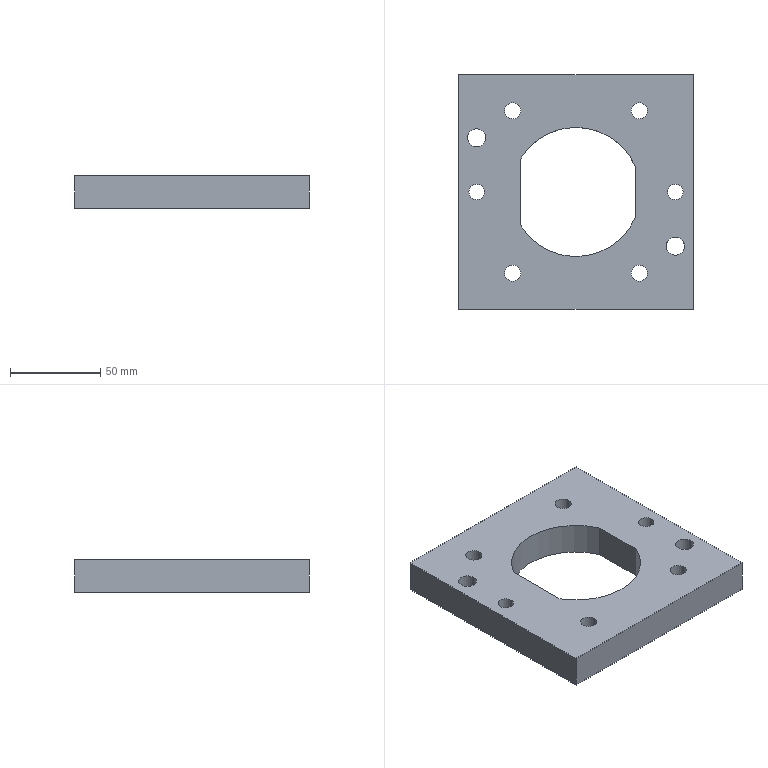Part | SolidWorks | features BaseBody 1 | 1 solid | 30 faces | box 130 x 130 x 18 mm | volume 225680 mm3 | cylinder 18 | plane 8 | cone 4 | commonest cylinder face diameters 9 x8 8.506 x4 10 x4 71.52 x2
STEP:
#1=CARTESIAN_POINT('',(-136.,5.,-28.7));
#2=VERTEX_POINT('',#1);
#3=CARTESIAN_POINT('',(-146.,5.,-28.7));
#4=VERTEX_POINT('',#3);
#5=CARTESIAN_POINT('',(-141.,5.,-28.7));
#6=DIRECTION('',(0.,0.,-1.));
#7=DIRECTION('',(-1.,0.,0.));
#8=AXIS2_PLACEMENT_3D('',#5,#6,#7);
#9=CIRCLE('',#8,5.);
#10=EDGE_CURVE('',#2,#4,#9,.T.);
#11=ORIENTED_EDGE('',*,*,#10,.F.);
#12=CARTESIAN_POINT('',(-136.,5.,-46.7));
#13=VERTEX_POINT('',#12);
#14=CARTESIAN_POINT('',(-136.,5.,-28.7));
#15=DIRECTION('',(0.,0.,-1.));
#16=VECTOR('',#15,1000.);
#17=LINE('',#14,#16);
#18=EDGE_CURVE('',#2,#13,#17,.T.);
#19=ORIENTED_EDGE('',*,*,#18,.T.);
#20=CARTESIAN_POINT('',(-146.,5.,-46.7));
#21=VERTEX_POINT('',#20);
#22=CARTESIAN_POINT('',(-141.,5.,-46.7));
#23=DIRECTION('',(0.,0.,-1.));
#24=DIRECTION('',(-1.,0.,0.));
#25=AXIS2_PLACEMENT_3D('',#22,#23,#24);
#26=CIRCLE('',#25,5.);
#27=EDGE_CURVE('',#13,#21,#26,.T.);
#28=ORIENTED_EDGE('',*,*,#27,.T.);
#29=CARTESIAN_POINT('',(-146.,5.,-28.7));
#30=DIRECTION('',(0.,0.,-1.));
#31=VECTOR('',#30,1000.);
#32=LINE('',#29,#31);
#33=EDGE_CURVE('',#4,#21,#32,.T.);
#34=ORIENTED_EDGE('',*,*,#33,.F.);
#35=EDGE_LOOP('',(#11,#19,#28,#34));
#36=FACE_OUTER_BOUND('',#35,.T.);
#37=CARTESIAN_POINT('',(-141.,5.,-28.7));
#38=DIRECTION('',(0.,0.,-1.));
#39=DIRECTION('',(-1.,0.,0.));
#40=AXIS2_PLACEMENT_3D('',#37,#38,#39);
#41=CYLINDRICAL_SURFACE('',#40,5.);
#42=ADVANCED_FACE('',(#36),#41,.F.);
#43=CARTESIAN_POINT('',(-26.,-55.,-28.7));
#44=VERTEX_POINT('',#43);
#45=CARTESIAN_POINT('',(-36.,-55.,-28.7));
#46=VERTEX_POINT('',#45);
#47=CARTESIAN_POINT('',(-31.,-55.,-28.7));
#48=DIRECTION('',(0.,0.,-1.));
#49=DIRECTION('',(-1.,0.,0.));
#50=AXIS2_PLACEMENT_3D('',#47,#48,#49);
#51=CIRCLE('',#50,5.);
#52=EDGE_CURVE('',#44,#46,#51,.T.);
#53=ORIENTED_EDGE('',*,*,#52,.F.);
#54=CARTESIAN_POINT('',(-26.,-55.,-46.7));
#55=VERTEX_POINT('',#54);
#56=CARTESIAN_POINT('',(-26.,-55.,-28.7));
#57=DIRECTION('',(0.,0.,-1.));
#58=VECTOR('',#57,1000.);
#59=LINE('',#56,#58);
#60=EDGE_CURVE('',#44,#55,#59,.T.);
#61=ORIENTED_EDGE('',*,*,#60,.T.);
#62=CARTESIAN_POINT('',(-36.,-55.,-46.7));
#63=VERTEX_POINT('',#62);
#64=CARTESIAN_POINT('',(-31.,-55.,-46.7));
#65=DIRECTION('',(0.,0.,-1.));
#66=DIRECTION('',(-1.,0.,0.));
#67=AXIS2_PLACEMENT_3D('',#64,#65,#66);
#68=CIRCLE('',#67,5.);
#69=EDGE_CURVE('',#55,#63,#68,.T.);
#70=ORIENTED_EDGE('',*,*,#69,.T.);
#71=CARTESIAN_POINT('',(-36.,-55.,-28.7));
#72=DIRECTION('',(0.,0.,-1.));
#73=VECTOR('',#72,1000.);
#74=LINE('',#71,#73);
#75=EDGE_CURVE('',#46,#63,#74,.T.);
#76=ORIENTED_EDGE('',*,*,#75,.F.);
#77=EDGE_LOOP('',(#53,#61,#70,#76));
#78=FACE_OUTER_BOUND('',#77,.T.);
#79=CARTESIAN_POINT('',(-31.,-55.,-28.7));
#80=DIRECTION('',(0.,0.,-1.));
#81=DIRECTION('',(-1.,0.,0.));
#82=AXIS2_PLACEMENT_3D('',#79,#80,#81);
#83=CYLINDRICAL_SURFACE('',#82,5.);
#84=ADVANCED_FACE('',(#78),#83,.F.);
#85=CARTESIAN_POINT('',(-145.253,-25.,-45.953));
#86=VERTEX_POINT('',#85);
#87=CARTESIAN_POINT('',(-136.747,-25.,-45.953));
#88=VERTEX_POINT('',#87);
#89=CARTESIAN_POINT('',(-141.,-25.,-45.953));
#90=DIRECTION('',(0.,0.,1.));
#91=DIRECTION('',(-1.,0.,0.));
#92=AXIS2_PLACEMENT_3D('',#89,#90,#91);
#93=CIRCLE('',#92,4.253);
#94=EDGE_CURVE('',#86,#88,#93,.T.);
#95=ORIENTED_EDGE('',*,*,#94,.T.);
#96=CARTESIAN_POINT('',(-136.,-25.,-46.7));
#97=VERTEX_POINT('',#96);
#98=CARTESIAN_POINT('',(-136.,-25.,-46.7));
#99=DIRECTION('',(0.7071,0.,-0.7071));
#100=VECTOR('',#99,1000.);
#101=LINE('',#98,#100);
#102=EDGE_CURVE('',#88,#97,#101,.T.);
#103=ORIENTED_EDGE('',*,*,#102,.T.);
#104=CARTESIAN_POINT('',(-146.,-25.,-46.7));
#105=VERTEX_POINT('',#104);
#106=CARTESIAN_POINT('',(-141.,-25.,-46.7));
#107=DIRECTION('',(0.,0.,-1.));
#108=DIRECTION('',(-1.,0.,0.));
#109=AXIS2_PLACEMENT_3D('',#106,#107,#108);
#110=CIRCLE('',#109,5.);
#111=EDGE_CURVE('',#97,#105,#110,.T.);
#112=ORIENTED_EDGE('',*,*,#111,.T.);
#113=CARTESIAN_POINT('',(-146.,-25.,-46.7));
#114=DIRECTION('',(-0.7071,0.,-0.7071));
#115=VECTOR('',#114,1000.);
#116=LINE('',#113,#115);
#117=EDGE_CURVE('',#86,#105,#116,.T.);
#118=ORIENTED_EDGE('',*,*,#117,.F.);
#119=EDGE_LOOP('',(#95,#103,#112,#118));
#120=FACE_OUTER_BOUND('',#119,.T.);
#121=CARTESIAN_POINT('',(-141.,-25.,-46.7));
#122=DIRECTION('',(0.,0.,-1.));
#123=DIRECTION('',(-1.,0.,0.));
#124=AXIS2_PLACEMENT_3D('',#121,#122,#123);
#125=CONICAL_SURFACE('',#124,5.,0.7854);
#126=ADVANCED_FACE('',(#120),#125,.F.);
#127=CARTESIAN_POINT('',(-136.747,-25.,-28.7));
#128=VERTEX_POINT('',#127);
#129=CARTESIAN_POINT('',(-145.253,-25.,-28.7));
#130=VERTEX_POINT('',#129);
#131=CARTESIAN_POINT('',(-141.,-25.,-28.7));
#132=DIRECTION('',(0.,0.,-1.));
#133=DIRECTION('',(-1.,0.,0.));
#134=AXIS2_PLACEMENT_3D('',#131,#132,#133);
#135=CIRCLE('',#134,4.253);
#136=EDGE_CURVE('',#128,#130,#135,.T.);
#137=ORIENTED_EDGE('',*,*,#136,.F.);
#138=CARTESIAN_POINT('',(-136.747,-25.,-11.867));
#139=DIRECTION('',(0.,0.,-1.));
#140=VECTOR('',#139,1000.);
#141=LINE('',#138,#140);
#142=EDGE_CURVE('',#128,#88,#141,.T.);
#143=ORIENTED_EDGE('',*,*,#142,.T.);
#144=ORIENTED_EDGE('',*,*,#94,.F.);
#145=CARTESIAN_POINT('',(-145.253,-25.,-11.867));
#146=DIRECTION('',(0.,0.,-1.));
#147=VECTOR('',#146,1000.);
#148=LINE('',#145,#147);
#149=EDGE_CURVE('',#130,#86,#148,.T.);
#150=ORIENTED_EDGE('',*,*,#149,.F.);
#151=EDGE_LOOP('',(#137,#143,#144,#150));
#152=FACE_OUTER_BOUND('',#151,.T.);
#153=CARTESIAN_POINT('',(-141.,-25.,-11.867));
#154=DIRECTION('',(0.,0.,-1.));
#155=DIRECTION('',(-1.,0.,0.));
#156=AXIS2_PLACEMENT_3D('',#153,#154,#155);
#157=CYLINDRICAL_SURFACE('',#156,4.253);
#158=ADVANCED_FACE('',(#152),#157,.F.);
#159=CARTESIAN_POINT('',(-35.253,-25.,-45.953));
#160=VERTEX_POINT('',#159);
#161=CARTESIAN_POINT('',(-26.747,-25.,-45.953));
#162=VERTEX_POINT('',#161);
#163=CARTESIAN_POINT('',(-31.,-25.,-45.953));
#164=DIRECTION('',(0.,0.,1.));
#165=DIRECTION('',(-1.,0.,0.));
#166=AXIS2_PLACEMENT_3D('',#163,#164,#165);
#167=CIRCLE('',#166,4.253);
#168=EDGE_CURVE('',#160,#162,#167,.T.);
#169=ORIENTED_EDGE('',*,*,#168,.T.);
#170=CARTESIAN_POINT('',(-26.,-25.,-46.7));
#171=VERTEX_POINT('',#170);
#172=CARTESIAN_POINT('',(-26.,-25.,-46.7));
#173=DIRECTION('',(0.7071,0.,-0.7071));
#174=VECTOR('',#173,1000.);
#175=LINE('',#172,#174);
#176=EDGE_CURVE('',#162,#171,#175,.T.);
#177=ORIENTED_EDGE('',*,*,#176,.T.);
#178=CARTESIAN_POINT('',(-36.,-25.,-46.7));
#179=VERTEX_POINT('',#178);
#180=CARTESIAN_POINT('',(-31.,-25.,-46.7));
#181=DIRECTION('',(0.,0.,-1.));
#182=DIRECTION('',(-1.,0.,0.));
#183=AXIS2_PLACEMENT_3D('',#180,#181,#182);
#184=CIRCLE('',#183,5.);
#185=EDGE_CURVE('',#171,#179,#184,.T.);
#186=ORIENTED_EDGE('',*,*,#185,.T.);
#187=CARTESIAN_POINT('',(-36.,-25.,-46.7));
#188=DIRECTION('',(-0.7071,0.,-0.7071));
#189=VECTOR('',#188,1000.);
#190=LINE('',#187,#189);
#191=EDGE_CURVE('',#160,#179,#190,.T.);
#192=ORIENTED_EDGE('',*,*,#191,.F.);
#193=EDGE_LOOP('',(#169,#177,#186,#192));
#194=FACE_OUTER_BOUND('',#193,.T.);
#195=CARTESIAN_POINT('',(-31.,-25.,-46.7));
#196=DIRECTION('',(0.,0.,-1.));
#197=DIRECTION('',(-1.,0.,0.));
#198=AXIS2_PLACEMENT_3D('',#195,#196,#197);
#199=CONICAL_SURFACE('',#198,5.,0.7854);
#200=ADVANCED_FACE('',(#194),#199,.F.);
#201=CARTESIAN_POINT('',(-26.747,-25.,-28.7));
#202=VERTEX_POINT('',#201);
#203=CARTESIAN_POINT('',(-35.253,-25.,-28.7));
#204=VERTEX_POINT('',#203);
#205=CARTESIAN_POINT('',(-31.,-25.,-28.7));
#206=DIRECTION('',(0.,0.,-1.));
#207=DIRECTION('',(-1.,0.,0.));
#208=AXIS2_PLACEMENT_3D('',#205,#206,#207);
#209=CIRCLE('',#208,4.253);
#210=EDGE_CURVE('',#202,#204,#209,.T.);
#211=ORIENTED_EDGE('',*,*,#210,.F.);
#212=CARTESIAN_POINT('',(-26.747,-25.,-11.867));
#213=DIRECTION('',(0.,0.,-1.));
#214=VECTOR('',#213,1000.);
#215=LINE('',#212,#214);
#216=EDGE_CURVE('',#202,#162,#215,.T.);
#217=ORIENTED_EDGE('',*,*,#216,.T.);
#218=ORIENTED_EDGE('',*,*,#168,.F.);
#219=CARTESIAN_POINT('',(-35.253,-25.,-11.867));
#220=DIRECTION('',(0.,0.,-1.));
#221=VECTOR('',#220,1000.);
#222=LINE('',#219,#221);
#223=EDGE_CURVE('',#204,#160,#222,.T.);
#224=ORIENTED_EDGE('',*,*,#223,.F.);
#225=EDGE_LOOP('',(#211,#217,#218,#224));
#226=FACE_OUTER_BOUND('',#225,.T.);
#227=CARTESIAN_POINT('',(-31.,-25.,-11.867));
#228=DIRECTION('',(0.,0.,-1.));
#229=DIRECTION('',(-1.,0.,0.));
#230=AXIS2_PLACEMENT_3D('',#227,#228,#229);
#231=CYLINDRICAL_SURFACE('',#230,4.253);
#232=ADVANCED_FACE('',(#226),#231,.F.);
#233=CARTESIAN_POINT('',(-125.5,-70.,-46.7));
#234=VERTEX_POINT('',#233);
#235=CARTESIAN_POINT('',(-116.5,-70.,-46.7));
#236=VERTEX_POINT('',#235);
#237=CARTESIAN_POINT('',(-121.,-70.,-46.7));
#238=DIRECTION('',(0.,0.,-1.));
#239=DIRECTION('',(-1.,0.,0.));
#240=AXIS2_PLACEMENT_3D('',#237,#238,#239);
#241=CIRCLE('',#240,4.5);
#242=EDGE_CURVE('',#234,#236,#241,.T.);
#243=ORIENTED_EDGE('',*,*,#242,.T.);
#244=CARTESIAN_POINT('',(-116.5,-70.,-28.7));
#245=VERTEX_POINT('',#244);
#246=CARTESIAN_POINT('',(-116.5,-70.,-51.7));
#247=DIRECTION('',(0.,0.,1.));
#248=VECTOR('',#247,1000.);
#249=LINE('',#246,#248);
#250=EDGE_CURVE('',#236,#245,#249,.T.);
#251=ORIENTED_EDGE('',*,*,#250,.T.);
#252=CARTESIAN_POINT('',(-125.5,-70.,-28.7));
#253=VERTEX_POINT('',#252);
#254=CARTESIAN_POINT('',(-121.,-70.,-28.7));
#255=DIRECTION('',(0.,0.,-1.));
#256=DIRECTION('',(-1.,0.,0.));
#257=AXIS2_PLACEMENT_3D('',#254,#255,#256);
#258=CIRCLE('',#257,4.5);
#259=EDGE_CURVE('',#253,#245,#258,.T.);
#260=ORIENTED_EDGE('',*,*,#259,.F.);
#261=CARTESIAN_POINT('',(-125.5,-70.,-51.7));
#262=DIRECTION('',(0.,0.,1.));
#263=VECTOR('',#262,1000.);
#264=LINE('',#261,#263);
#265=EDGE_CURVE('',#234,#253,#264,.T.);
#266=ORIENTED_EDGE('',*,*,#265,.F.);
#267=EDGE_LOOP('',(#243,#251,#260,#266));
#268=FACE_OUTER_BOUND('',#267,.T.);
#269=CARTESIAN_POINT('',(-121.,-70.,-51.7));
#270=DIRECTION('',(0.,0.,1.));
#271=DIRECTION('',(-1.,0.,0.));
#272=AXIS2_PLACEMENT_3D('',#269,#270,#271);
#273=CYLINDRICAL_SURFACE('',#272,4.5);
#274=ADVANCED_FACE('',(#268),#273,.F.);
#275=CARTESIAN_POINT('',(-46.5,20.,-46.7));
#276=VERTEX_POINT('',#275);
#277=CARTESIAN_POINT('',(-55.5,20.,-46.7));
#278=VERTEX_POINT('',#277);
#279=CARTESIAN_POINT('',(-51.,20.,-46.7));
#280=DIRECTION('',(0.,0.,-1.));
#281=DIRECTION('',(-1.,0.,0.));
#282=AXIS2_PLACEMENT_3D('',#279,#280,#281);
#283=CIRCLE('',#282,4.5);
#284=EDGE_CURVE('',#276,#278,#283,.T.);
#285=ORIENTED_EDGE('',*,*,#284,.T.);
#286=CARTESIAN_POINT('',(-55.5,20.,-28.7));
#287=VERTEX_POINT('',#286);
#288=CARTESIAN_POINT('',(-55.5,20.,-51.7));
#289=DIRECTION('',(0.,0.,1.));
#290=VECTOR('',#289,1000.);
#291=LINE('',#288,#290);
#292=EDGE_CURVE('',#278,#287,#291,.T.);
#293=ORIENTED_EDGE('',*,*,#292,.T.);
#294=CARTESIAN_POINT('',(-46.5,20.,-28.7));
#295=VERTEX_POINT('',#294);
#296=CARTESIAN_POINT('',(-51.,20.,-28.7));
#297=DIRECTION('',(0.,0.,-1.));
#298=DIRECTION('',(-1.,0.,0.));
#299=AXIS2_PLACEMENT_3D('',#296,#297,#298);
#300=CIRCLE('',#299,4.5);
#301=EDGE_CURVE('',#295,#287,#300,.T.);
#302=ORIENTED_EDGE('',*,*,#301,.F.);
#303=CARTESIAN_POINT('',(-46.5,20.,-51.7));
#304=DIRECTION('',(0.,0.,1.));
#305=VECTOR('',#304,1000.);
#306=LINE('',#303,#305);
#307=EDGE_CURVE('',#276,#295,#306,.T.);
#308=ORIENTED_EDGE('',*,*,#307,.F.);
#309=EDGE_LOOP('',(#285,#293,#302,#308));
#310=FACE_OUTER_BOUND('',#309,.T.);
#311=CARTESIAN_POINT('',(-51.,20.,-51.7));
#312=DIRECTION('',(0.,0.,1.));
#313=DIRECTION('',(1.,0.,0.));
#314=AXIS2_PLACEMENT_3D('',#311,#312,#313);
#315=CYLINDRICAL_SURFACE('',#314,4.5);
#316=ADVANCED_FACE('',(#310),#315,.F.);
#317=CARTESIAN_POINT('',(-116.5,20.,-46.7));
#318=VERTEX_POINT('',#317);
#319=CARTESIAN_POINT('',(-125.5,20.,-46.7));
#320=VERTEX_POINT('',#319);
#321=CARTESIAN_POINT('',(-121.,20.,-46.7));
#322=DIRECTION('',(0.,0.,1.));
#323=DIRECTION('',(-1.,0.,0.));
#324=AXIS2_PLACEMENT_3D('',#321,#322,#323);
#325=CIRCLE('',#324,4.5);
#326=EDGE_CURVE('',#318,#320,#325,.T.);
#327=ORIENTED_EDGE('',*,*,#326,.F.);
#328=CARTESIAN_POINT('',(-116.5,20.,-28.7));
#329=VERTEX_POINT('',#328);
#330=CARTESIAN_POINT('',(-116.5,20.,-51.7));
#331=DIRECTION('',(0.,0.,1.));
#332=VECTOR('',#331,1000.);
#333=LINE('',#330,#332);
#334=EDGE_CURVE('',#318,#329,#333,.T.);
#335=ORIENTED_EDGE('',*,*,#334,.T.);
#336=CARTESIAN_POINT('',(-125.5,20.,-28.7));
#337=VERTEX_POINT('',#336);
#338=CARTESIAN_POINT('',(-121.,20.,-28.7));
#339=DIRECTION('',(0.,0.,-1.));
#340=DIRECTION('',(-1.,0.,0.));
#341=AXIS2_PLACEMENT_3D('',#338,#339,#340);
#342=CIRCLE('',#341,4.5);
#343=EDGE_CURVE('',#337,#329,#342,.T.);
#344=ORIENTED_EDGE('',*,*,#343,.F.);
#345=CARTESIAN_POINT('',(-125.5,20.,-51.7));
#346=DIRECTION('',(0.,0.,1.));
#347=VECTOR('',#346,1000.);
#348=LINE('',#345,#347);
#349=EDGE_CURVE('',#320,#337,#348,.T.);
#350=ORIENTED_EDGE('',*,*,#349,.F.);
#351=EDGE_LOOP('',(#327,#335,#344,#350));
#352=FACE_OUTER_BOUND('',#351,.T.);
#353=CARTESIAN_POINT('',(-121.,20.,-51.7));
#354=DIRECTION('',(0.,0.,1.));
#355=DIRECTION('',(-1.,0.,0.));
#356=AXIS2_PLACEMENT_3D('',#353,#354,#355);
#357=CYLINDRICAL_SURFACE('',#356,4.5);
#358=ADVANCED_FACE('',(#352),#357,.F.);
#359=CARTESIAN_POINT('',(-55.5,-70.,-46.7));
#360=VERTEX_POINT('',#359);
#361=CARTESIAN_POINT('',(-46.5,-70.,-46.7));
#362=VERTEX_POINT('',#361);
#363=CARTESIAN_POINT('',(-51.,-70.,-46.7));
#364=DIRECTION('',(0.,0.,1.));
#365=DIRECTION('',(-1.,0.,0.));
#366=AXIS2_PLACEMENT_3D('',#363,#364,#365);
#367=CIRCLE('',#366,4.5);
#368=EDGE_CURVE('',#360,#362,#367,.T.);
#369=ORIENTED_EDGE('',*,*,#368,.F.);
#370=CARTESIAN_POINT('',(-55.5,-70.,-28.7));
#371=VERTEX_POINT('',#370);
#372=CARTESIAN_POINT('',(-55.5,-70.,-51.7));
#373=DIRECTION('',(0.,0.,1.));
#374=VECTOR('',#373,1000.);
#375=LINE('',#372,#374);
#376=EDGE_CURVE('',#360,#371,#375,.T.);
#377=ORIENTED_EDGE('',*,*,#376,.T.);
#378=CARTESIAN_POINT('',(-46.5,-70.,-28.7));
#379=VERTEX_POINT('',#378);
#380=CARTESIAN_POINT('',(-51.,-70.,-28.7));
#381=DIRECTION('',(0.,0.,-1.));
#382=DIRECTION('',(-1.,0.,0.));
#383=AXIS2_PLACEMENT_3D('',#380,#381,#382);
#384=CIRCLE('',#383,4.5);
#385=EDGE_CURVE('',#379,#371,#384,.T.);
#386=ORIENTED_EDGE('',*,*,#385,.F.);
#387=CARTESIAN_POINT('',(-46.5,-70.,-51.7));
#388=DIRECTION('',(0.,0.,1.));
#389=VECTOR('',#388,1000.);
#390=LINE('',#387,#389);
#391=EDGE_CURVE('',#362,#379,#390,.T.);
#392=ORIENTED_EDGE('',*,*,#391,.F.);
#393=EDGE_LOOP('',(#369,#377,#386,#392));
#394=FACE_OUTER_BOUND('',#393,.T.);
#395=CARTESIAN_POINT('',(-51.,-70.,-51.7));
#396=DIRECTION('',(0.,0.,1.));
#397=DIRECTION('',(1.,0.,0.));
#398=AXIS2_PLACEMENT_3D('',#395,#396,#397);
#399=CYLINDRICAL_SURFACE('',#398,4.5);
#400=ADVANCED_FACE('',(#394),#399,.F.);
#401=CARTESIAN_POINT('',(-141.,5.,-46.7));
#402=DIRECTION('',(0.,0.,-1.));
#403=DIRECTION('',(-1.,0.,0.));
#404=AXIS2_PLACEMENT_3D('',#401,#402,#403);
#405=CIRCLE('',#404,5.);
#406=EDGE_CURVE('',#21,#13,#405,.T.);
#407=ORIENTED_EDGE('',*,*,#406,.F.);
#408=ORIENTED_EDGE('',*,*,#27,.F.);
#409=EDGE_LOOP('',(#407,#408));
#410=FACE_BOUND('',#409,.T.);
#411=CARTESIAN_POINT('',(-151.,-90.,-46.7));
#412=VERTEX_POINT('',#411);
#413=CARTESIAN_POINT('',(-21.,-90.,-46.7));
#414=VERTEX_POINT('',#413);
#415=CARTESIAN_POINT('',(-86.,-90.,-46.7));
#416=DIRECTION('',(1.,0.,0.));
#417=VECTOR('',#416,1000.);
#418=LINE('',#415,#417);
#419=EDGE_CURVE('',#412,#414,#418,.T.);
#420=ORIENTED_EDGE('',*,*,#419,.F.);
#421=CARTESIAN_POINT('',(-151.,40.,-46.7));
#422=VERTEX_POINT('',#421);
#423=CARTESIAN_POINT('',(-151.,-25.,-46.7));
#424=DIRECTION('',(0.,-1.,0.));
#425=VECTOR('',#424,1000.);
#426=LINE('',#423,#425);
#427=EDGE_CURVE('',#422,#412,#426,.T.);
#428=ORIENTED_EDGE('',*,*,#427,.F.);
#429=CARTESIAN_POINT('',(-21.,40.,-46.7));
#430=VERTEX_POINT('',#429);
#431=CARTESIAN_POINT('',(-86.,40.,-46.7));
#432=DIRECTION('',(-1.,0.,0.));
#433=VECTOR('',#432,1000.);
#434=LINE('',#431,#433);
#435=EDGE_CURVE('',#430,#422,#434,.T.);
#436=ORIENTED_EDGE('',*,*,#435,.F.);
#437=CARTESIAN_POINT('',(-21.,-25.,-46.7));
#438=DIRECTION('',(0.,1.,0.));
#439=VECTOR('',#438,1000.);
#440=LINE('',#437,#439);
#441=EDGE_CURVE('',#414,#430,#440,.T.);
#442=ORIENTED_EDGE('',*,*,#441,.F.);
#443=EDGE_LOOP('',(#420,#428,#436,#442));
#444=FACE_OUTER_BOUND('',#443,.T.);
#445=CARTESIAN_POINT('',(-31.,-55.,-46.7));
#446=DIRECTION('',(0.,0.,-1.));
#447=DIRECTION('',(-1.,0.,0.));
#448=AXIS2_PLACEMENT_3D('',#445,#446,#447);
#449=CIRCLE('',#448,5.);
#450=EDGE_CURVE('',#63,#55,#449,.T.);
#451=ORIENTED_EDGE('',*,*,#450,.F.);
#452=ORIENTED_EDGE('',*,*,#69,.F.);
#453=EDGE_LOOP('',(#451,#452));
#454=FACE_BOUND('',#453,.T.);
#455=CARTESIAN_POINT('',(-141.,-25.,-46.7));
#456=DIRECTION('',(0.,0.,-1.));
#457=DIRECTION('',(-1.,0.,0.));
#458=AXIS2_PLACEMENT_3D('',#455,#456,#457);
#459=CIRCLE('',#458,5.);
#460=EDGE_CURVE('',#105,#97,#459,.T.);
#461=ORIENTED_EDGE('',*,*,#460,.F.);
#462=ORIENTED_EDGE('',*,*,#111,.F.);
#463=EDGE_LOOP('',(#461,#462));
#464=FACE_BOUND('',#463,.T.);
#465=CARTESIAN_POINT('',(-31.,-25.,-46.7));
#466=DIRECTION('',(0.,0.,-1.));
#467=DIRECTION('',(-1.,0.,0.));
#468=AXIS2_PLACEMENT_3D('',#465,#466,#467);
#469=CIRCLE('',#468,5.);
#470=EDGE_CURVE('',#179,#171,#469,.T.);
#471=ORIENTED_EDGE('',*,*,#470,.F.);
#472=ORIENTED_EDGE('',*,*,#185,.F.);
#473=EDGE_LOOP('',(#471,#472));
#474=FACE_BOUND('',#473,.T.);
#475=CARTESIAN_POINT('',(-53.24,-10.663,-46.7));
#476=VERTEX_POINT('',#475);
#477=CARTESIAN_POINT('',(-116.76,-6.763,-46.7));
#478=VERTEX_POINT('',#477);
#479=CARTESIAN_POINT('',(-86.,-25.,-46.7));
#480=DIRECTION('',(0.,0.,1.));
#481=DIRECTION('',(-1.,0.,0.));
#482=AXIS2_PLACEMENT_3D('',#479,#480,#481);
#483=CIRCLE('',#482,35.76);
#484=EDGE_CURVE('',#476,#478,#483,.T.);
#485=ORIENTED_EDGE('',*,*,#484,.T.);
#486=CARTESIAN_POINT('',(-116.76,-43.237,-46.7));
#487=VERTEX_POINT('',#486);
#488=CARTESIAN_POINT('',(-116.76,-25.,-46.7));
#489=DIRECTION('',(0.,-1.,0.));
#490=VECTOR('',#489,1000.);
#491=LINE('',#488,#490);
#492=EDGE_CURVE('',#478,#487,#491,.T.);
#493=ORIENTED_EDGE('',*,*,#492,.T.);
#494=CARTESIAN_POINT('',(-53.24,-39.337,-46.7));
#495=VERTEX_POINT('',#494);
#496=CARTESIAN_POINT('',(-86.,-25.,-46.7));
#497=DIRECTION('',(0.,0.,1.));
#498=DIRECTION('',(-1.,0.,0.));
#499=AXIS2_PLACEMENT_3D('',#496,#497,#498);
#500=CIRCLE('',#499,35.76);
#501=EDGE_CURVE('',#487,#495,#500,.T.);
#502=ORIENTED_EDGE('',*,*,#501,.T.);
#503=CARTESIAN_POINT('',(-53.24,-25.,-46.7));
#504=DIRECTION('',(0.,1.,0.));
#505=VECTOR('',#504,1000.);
#506=LINE('',#503,#505);
#507=EDGE_CURVE('',#495,#476,#506,.T.);
#508=ORIENTED_EDGE('',*,*,#507,.T.);
#509=EDGE_LOOP('',(#485,#493,#502,#508));
#510=FACE_BOUND('',#509,.T.);
#511=CARTESIAN_POINT('',(-51.,-70.,-46.7));
#512=DIRECTION('',(0.,0.,1.));
#513=DIRECTION('',(-1.,0.,0.));
#514=AXIS2_PLACEMENT_3D('',#511,#512,#513);
#515=CIRCLE('',#514,4.5);
#516=EDGE_CURVE('',#362,#360,#515,.T.);
#517=ORIENTED_EDGE('',*,*,#516,.T.);
#518=ORIENTED_EDGE('',*,*,#368,.T.);
#519=EDGE_LOOP('',(#517,#518));
#520=FACE_BOUND('',#519,.T.);
#521=ORIENTED_EDGE('',*,*,#284,.F.);
#522=CARTESIAN_POINT('',(-51.,20.,-46.7));
#523=DIRECTION('',(0.,0.,-1.));
#524=DIRECTION('',(-1.,0.,0.));
#525=AXIS2_PLACEMENT_3D('',#522,#523,#524);
#526=CIRCLE('',#525,4.5);
#527=EDGE_CURVE('',#278,#276,#526,.T.);
#528=ORIENTED_EDGE('',*,*,#527,.F.);
#529=EDGE_LOOP('',(#521,#528));
#530=FACE_BOUND('',#529,.T.);
#531=CARTESIAN_POINT('',(-121.,20.,-46.7));
#532=DIRECTION('',(0.,0.,1.));
#533=DIRECTION('',(-1.,0.,0.));
#534=AXIS2_PLACEMENT_3D('',#531,#532,#533);
#535=CIRCLE('',#534,4.5);
#536=EDGE_CURVE('',#320,#318,#535,.T.);
#537=ORIENTED_EDGE('',*,*,#536,.T.);
#538=ORIENTED_EDGE('',*,*,#326,.T.);
#539=EDGE_LOOP('',(#537,#538));
#540=FACE_BOUND('',#539,.T.);
#541=ORIENTED_EDGE('',*,*,#242,.F.);
#542=CARTESIAN_POINT('',(-121.,-70.,-46.7));
#543=DIRECTION('',(0.,0.,-1.));
#544=DIRECTION('',(-1.,0.,0.));
#545=AXIS2_PLACEMENT_3D('',#542,#543,#544);
#546=CIRCLE('',#545,4.5);
#547=EDGE_CURVE('',#236,#234,#546,.T.);
#548=ORIENTED_EDGE('',*,*,#547,.F.);
#549=EDGE_LOOP('',(#541,#548));
#550=FACE_BOUND('',#549,.T.);
#551=CARTESIAN_POINT('',(-86.,-25.,-46.7));
#552=DIRECTION('',(0.,0.,-1.));
#553=DIRECTION('',(-1.,0.,0.));
#554=AXIS2_PLACEMENT_3D('',#551,#552,#553);
#555=PLANE('',#554);
#556=ADVANCED_FACE('',(#410,#444,#454,#464,#474,#510,#520,#530,#540,#550),#555,.T.);
#557=CARTESIAN_POINT('',(-151.,-90.,-28.7));
#558=VERTEX_POINT('',#557);
#559=CARTESIAN_POINT('',(-21.,-90.,-28.7));
#560=VERTEX_POINT('',#559);
#561=CARTESIAN_POINT('',(-86.,-90.,-28.7));
#562=DIRECTION('',(1.,0.,0.));
#563=VECTOR('',#562,1000.);
#564=LINE('',#561,#563);
#565=EDGE_CURVE('',#558,#560,#564,.T.);
#566=ORIENTED_EDGE('',*,*,#565,.F.);
#567=CARTESIAN_POINT('',(-151.,-90.,-8.7));
#568=DIRECTION('',(0.,0.,-1.));
#569=VECTOR('',#568,1000.);
#570=LINE('',#567,#569);
#571=EDGE_CURVE('',#558,#412,#570,.T.);
#572=ORIENTED_EDGE('',*,*,#571,.T.);
#573=ORIENTED_EDGE('',*,*,#419,.T.);
#574=CARTESIAN_POINT('',(-21.,-90.,-8.7));
#575=DIRECTION('',(0.,0.,-1.));
#576=VECTOR('',#575,1000.);
#577=LINE('',#574,#576);
#578=EDGE_CURVE('',#560,#414,#577,.T.);
#579=ORIENTED_EDGE('',*,*,#578,.F.);
#580=EDGE_LOOP('',(#566,#572,#573,#579));
#581=FACE_OUTER_BOUND('',#580,.T.);
#582=CARTESIAN_POINT('',(-86.,-90.,-8.7));
#583=DIRECTION('',(0.,-1.,0.));
#584=DIRECTION('',(0.,0.,1.));
#585=AXIS2_PLACEMENT_3D('',#582,#583,#584);
#586=PLANE('',#585);
#587=ADVANCED_FACE('',(#581),#586,.T.);
#588=CARTESIAN_POINT('',(-21.,40.,-28.7));
#589=VERTEX_POINT('',#588);
#590=CARTESIAN_POINT('',(-21.,-25.,-28.7));
#591=DIRECTION('',(0.,1.,0.));
#592=VECTOR('',#591,1000.);
#593=LINE('',#590,#592);
#594=EDGE_CURVE('',#560,#589,#593,.T.);
#595=ORIENTED_EDGE('',*,*,#594,.F.);
#596=ORIENTED_EDGE('',*,*,#578,.T.);
#597=ORIENTED_EDGE('',*,*,#441,.T.);
#598=CARTESIAN_POINT('',(-21.,40.,-8.7));
#599=DIRECTION('',(0.,0.,-1.));
#600=VECTOR('',#599,1000.);
#601=LINE('',#598,#600);
#602=EDGE_CURVE('',#589,#430,#601,.T.);
#603=ORIENTED_EDGE('',*,*,#602,.F.);
#604=EDGE_LOOP('',(#595,#596,#597,#603));
#605=FACE_OUTER_BOUND('',#604,.T.);
#606=CARTESIAN_POINT('',(-21.,-25.,-8.7));
#607=DIRECTION('',(1.,0.,0.));
#608=DIRECTION('',(0.,0.,-1.));
#609=AXIS2_PLACEMENT_3D('',#606,#607,#608);
#610=PLANE('',#609);
#611=ADVANCED_FACE('',(#605),#610,.T.);
#612=CARTESIAN_POINT('',(-151.,40.,-28.7));
#613=VERTEX_POINT('',#612);
#614=CARTESIAN_POINT('',(-86.,40.,-28.7));
#615=DIRECTION('',(-1.,0.,0.));
#616=VECTOR('',#615,1000.);
#617=LINE('',#614,#616);
#618=EDGE_CURVE('',#589,#613,#617,.T.);
#619=ORIENTED_EDGE('',*,*,#618,.F.);
#620=ORIENTED_EDGE('',*,*,#602,.T.);
#621=ORIENTED_EDGE('',*,*,#435,.T.);
#622=CARTESIAN_POINT('',(-151.,40.,-8.7));
#623=DIRECTION('',(0.,0.,-1.));
#624=VECTOR('',#623,1000.);
#625=LINE('',#622,#624);
#626=EDGE_CURVE('',#613,#422,#625,.T.);
#627=ORIENTED_EDGE('',*,*,#626,.F.);
#628=EDGE_LOOP('',(#619,#620,#621,#627));
#629=FACE_OUTER_BOUND('',#628,.T.);
#630=CARTESIAN_POINT('',(-86.,40.,-8.7));
#631=DIRECTION('',(0.,1.,0.));
#632=DIRECTION('',(0.,0.,-1.));
#633=AXIS2_PLACEMENT_3D('',#630,#631,#632);
#634=PLANE('',#633);
#635=ADVANCED_FACE('',(#629),#634,.T.);
#636=CARTESIAN_POINT('',(-151.,-25.,-28.7));
#637=DIRECTION('',(0.,-1.,0.));
#638=VECTOR('',#637,1000.);
#639=LINE('',#636,#638);
#640=EDGE_CURVE('',#613,#558,#639,.T.);
#641=ORIENTED_EDGE('',*,*,#640,.F.);
#642=ORIENTED_EDGE('',*,*,#626,.T.);
#643=ORIENTED_EDGE('',*,*,#427,.T.);
#644=ORIENTED_EDGE('',*,*,#571,.F.);
#645=EDGE_LOOP('',(#641,#642,#643,#644));
#646=FACE_OUTER_BOUND('',#645,.T.);
#647=CARTESIAN_POINT('',(-151.,-25.,-8.7));
#648=DIRECTION('',(-1.,0.,0.));
#649=DIRECTION('',(0.,0.,1.));
#650=AXIS2_PLACEMENT_3D('',#647,#648,#649);
#651=PLANE('',#650);
#652=ADVANCED_FACE('',(#646),#651,.T.);
#653=ORIENTED_EDGE('',*,*,#618,.T.);
#654=ORIENTED_EDGE('',*,*,#640,.T.);
#655=ORIENTED_EDGE('',*,*,#565,.T.);
#656=ORIENTED_EDGE('',*,*,#594,.T.);
#657=EDGE_LOOP('',(#653,#654,#655,#656));
#658=FACE_OUTER_BOUND('',#657,.T.);
#659=CARTESIAN_POINT('',(-31.,-55.,-28.7));
#660=DIRECTION('',(0.,0.,-1.));
#661=DIRECTION('',(-1.,0.,0.));
#662=AXIS2_PLACEMENT_3D('',#659,#660,#661);
#663=CIRCLE('',#662,5.);
#664=EDGE_CURVE('',#46,#44,#663,.T.);
#665=ORIENTED_EDGE('',*,*,#664,.T.);
#666=ORIENTED_EDGE('',*,*,#52,.T.);
#667=EDGE_LOOP('',(#665,#666));
#668=FACE_BOUND('',#667,.T.);
#669=CARTESIAN_POINT('',(-141.,-25.,-28.7));
#670=DIRECTION('',(0.,0.,-1.));
#671=DIRECTION('',(-1.,0.,0.));
#672=AXIS2_PLACEMENT_3D('',#669,#670,#671);
#673=CIRCLE('',#672,4.253);
#674=EDGE_CURVE('',#130,#128,#673,.T.);
#675=ORIENTED_EDGE('',*,*,#674,.T.);
#676=ORIENTED_EDGE('',*,*,#136,.T.);
#677=EDGE_LOOP('',(#675,#676));
#678=FACE_BOUND('',#677,.T.);
#679=CARTESIAN_POINT('',(-31.,-25.,-28.7));
#680=DIRECTION('',(0.,0.,-1.));
#681=DIRECTION('',(-1.,0.,0.));
#682=AXIS2_PLACEMENT_3D('',#679,#680,#681);
#683=CIRCLE('',#682,4.253);
#684=EDGE_CURVE('',#204,#202,#683,.T.);
#685=ORIENTED_EDGE('',*,*,#684,.T.);
#686=ORIENTED_EDGE('',*,*,#210,.T.);
#687=EDGE_LOOP('',(#685,#686));
#688=FACE_BOUND('',#687,.T.);
#689=ORIENTED_EDGE('',*,*,#259,.T.);
#690=CARTESIAN_POINT('',(-121.,-70.,-28.7));
#691=DIRECTION('',(0.,0.,-1.));
#692=DIRECTION('',(-1.,0.,0.));
#693=AXIS2_PLACEMENT_3D('',#690,#691,#692);
#694=CIRCLE('',#693,4.5);
#695=EDGE_CURVE('',#245,#253,#694,.T.);
#696=ORIENTED_EDGE('',*,*,#695,.T.);
#697=EDGE_LOOP('',(#689,#696));
#698=FACE_BOUND('',#697,.T.);
#699=ORIENTED_EDGE('',*,*,#301,.T.);
#700=CARTESIAN_POINT('',(-51.,20.,-28.7));
#701=DIRECTION('',(0.,0.,-1.));
#702=DIRECTION('',(-1.,0.,0.));
#703=AXIS2_PLACEMENT_3D('',#700,#701,#702);
#704=CIRCLE('',#703,4.5);
#705=EDGE_CURVE('',#287,#295,#704,.T.);
#706=ORIENTED_EDGE('',*,*,#705,.T.);
#707=EDGE_LOOP('',(#699,#706));
#708=FACE_BOUND('',#707,.T.);
#709=ORIENTED_EDGE('',*,*,#343,.T.);
#710=CARTESIAN_POINT('',(-121.,20.,-28.7));
#711=DIRECTION('',(0.,0.,-1.));
#712=DIRECTION('',(-1.,0.,0.));
#713=AXIS2_PLACEMENT_3D('',#710,#711,#712);
#714=CIRCLE('',#713,4.5);
#715=EDGE_CURVE('',#329,#337,#714,.T.);
#716=ORIENTED_EDGE('',*,*,#715,.T.);
#717=EDGE_LOOP('',(#709,#716));
#718=FACE_BOUND('',#717,.T.);
#719=ORIENTED_EDGE('',*,*,#385,.T.);
#720=CARTESIAN_POINT('',(-51.,-70.,-28.7));
#721=DIRECTION('',(0.,0.,-1.));
#722=DIRECTION('',(-1.,0.,0.));
#723=AXIS2_PLACEMENT_3D('',#720,#721,#722);
#724=CIRCLE('',#723,4.5);
#725=EDGE_CURVE('',#371,#379,#724,.T.);
#726=ORIENTED_EDGE('',*,*,#725,.T.);
#727=EDGE_LOOP('',(#719,#726));
#728=FACE_BOUND('',#727,.T.);
#729=CARTESIAN_POINT('',(-53.24,-39.337,-28.7));
#730=VERTEX_POINT('',#729);
#731=CARTESIAN_POINT('',(-116.76,-43.237,-28.7));
#732=VERTEX_POINT('',#731);
#733=CARTESIAN_POINT('',(-86.,-25.,-28.7));
#734=DIRECTION('',(0.,0.,-1.));
#735=DIRECTION('',(-1.,0.,0.));
#736=AXIS2_PLACEMENT_3D('',#733,#734,#735);
#737=CIRCLE('',#736,35.76);
#738=EDGE_CURVE('',#730,#732,#737,.T.);
#739=ORIENTED_EDGE('',*,*,#738,.T.);
#740=CARTESIAN_POINT('',(-116.76,-6.763,-28.7));
#741=VERTEX_POINT('',#740);
#742=CARTESIAN_POINT('',(-116.76,-25.,-28.7));
#743=DIRECTION('',(0.,1.,0.));
#744=VECTOR('',#743,1000.);
#745=LINE('',#742,#744);
#746=EDGE_CURVE('',#732,#741,#745,.T.);
#747=ORIENTED_EDGE('',*,*,#746,.T.);
#748=CARTESIAN_POINT('',(-53.24,-10.663,-28.7));
#749=VERTEX_POINT('',#748);
#750=CARTESIAN_POINT('',(-86.,-25.,-28.7));
#751=DIRECTION('',(0.,0.,-1.));
#752=DIRECTION('',(-1.,0.,0.));
#753=AXIS2_PLACEMENT_3D('',#750,#751,#752);
#754=CIRCLE('',#753,35.76);
#755=EDGE_CURVE('',#741,#749,#754,.T.);
#756=ORIENTED_EDGE('',*,*,#755,.T.);
#757=CARTESIAN_POINT('',(-53.24,-25.,-28.7));
#758=DIRECTION('',(0.,-1.,0.));
#759=VECTOR('',#758,1000.);
#760=LINE('',#757,#759);
#761=EDGE_CURVE('',#749,#730,#760,.T.);
#762=ORIENTED_EDGE('',*,*,#761,.T.);
#763=EDGE_LOOP('',(#739,#747,#756,#762));
#764=FACE_BOUND('',#763,.T.);
#765=CARTESIAN_POINT('',(-141.,5.,-28.7));
#766=DIRECTION('',(0.,0.,-1.));
#767=DIRECTION('',(-1.,0.,0.));
#768=AXIS2_PLACEMENT_3D('',#765,#766,#767);
#769=CIRCLE('',#768,5.);
#770=EDGE_CURVE('',#4,#2,#769,.T.);
#771=ORIENTED_EDGE('',*,*,#770,.T.);
#772=ORIENTED_EDGE('',*,*,#10,.T.);
#773=EDGE_LOOP('',(#771,#772));
#774=FACE_BOUND('',#773,.T.);
#775=CARTESIAN_POINT('',(-86.,-25.,-28.7));
#776=DIRECTION('',(0.,0.,-1.));
#777=DIRECTION('',(-1.,0.,0.));
#778=AXIS2_PLACEMENT_3D('',#775,#776,#777);
#779=PLANE('',#778);
#780=ADVANCED_FACE('',(#658,#668,#678,#688,#698,#708,#718,#728,#764,#774),#779,.F.);
#781=CARTESIAN_POINT('',(-116.76,-6.763,-28.7));
#782=DIRECTION('',(0.,0.,-1.));
#783=VECTOR('',#782,1000.);
#784=LINE('',#781,#783);
#785=EDGE_CURVE('',#741,#478,#784,.T.);
#786=ORIENTED_EDGE('',*,*,#785,.T.);
#787=ORIENTED_EDGE('',*,*,#484,.F.);
#788=CARTESIAN_POINT('',(-53.24,-10.663,-46.7));
#789=DIRECTION('',(0.,0.,1.));
#790=VECTOR('',#789,1000.);
#791=LINE('',#788,#790);
#792=EDGE_CURVE('',#476,#749,#791,.T.);
#793=ORIENTED_EDGE('',*,*,#792,.T.);
#794=ORIENTED_EDGE('',*,*,#755,.F.);
#795=EDGE_LOOP('',(#786,#787,#793,#794));
#796=FACE_OUTER_BOUND('',#795,.T.);
#797=CARTESIAN_POINT('',(-86.,-25.,121.4));
#798=DIRECTION('',(0.,0.,-1.));
#799=DIRECTION('',(-1.,0.,0.));
#800=AXIS2_PLACEMENT_3D('',#797,#798,#799);
#801=CYLINDRICAL_SURFACE('',#800,35.76);
#802=ADVANCED_FACE('',(#796),#801,.F.);
#803=CARTESIAN_POINT('',(-53.24,-39.337,-28.7));
#804=DIRECTION('',(0.,0.,-1.));
#805=VECTOR('',#804,1000.);
#806=LINE('',#803,#805);
#807=EDGE_CURVE('',#730,#495,#806,.T.);
#808=ORIENTED_EDGE('',*,*,#807,.T.);
#809=ORIENTED_EDGE('',*,*,#501,.F.);
#810=CARTESIAN_POINT('',(-116.76,-43.237,-46.7));
#811=DIRECTION('',(0.,0.,1.));
#812=VECTOR('',#811,1000.);
#813=LINE('',#810,#812);
#814=EDGE_CURVE('',#487,#732,#813,.T.);
#815=ORIENTED_EDGE('',*,*,#814,.T.);
#816=ORIENTED_EDGE('',*,*,#738,.F.);
#817=EDGE_LOOP('',(#808,#809,#815,#816));
#818=FACE_OUTER_BOUND('',#817,.T.);
#819=CARTESIAN_POINT('',(-86.,-25.,121.4));
#820=DIRECTION('',(0.,0.,-1.));
#821=DIRECTION('',(-1.,0.,0.));
#822=AXIS2_PLACEMENT_3D('',#819,#820,#821);
#823=CYLINDRICAL_SURFACE('',#822,35.76);
#824=ADVANCED_FACE('',(#818),#823,.F.);
#825=ORIENTED_EDGE('',*,*,#814,.F.);
#826=ORIENTED_EDGE('',*,*,#492,.F.);
#827=ORIENTED_EDGE('',*,*,#785,.F.);
#828=ORIENTED_EDGE('',*,*,#746,.F.);
#829=EDGE_LOOP('',(#825,#826,#827,#828));
#830=FACE_OUTER_BOUND('',#829,.T.);
#831=CARTESIAN_POINT('',(-116.76,-25.,-46.7));
#832=DIRECTION('',(-1.,0.,0.));
#833=DIRECTION('',(0.,0.,1.));
#834=AXIS2_PLACEMENT_3D('',#831,#832,#833);
#835=PLANE('',#834);
#836=ADVANCED_FACE('',(#830),#835,.F.);
#837=ORIENTED_EDGE('',*,*,#792,.F.);
#838=ORIENTED_EDGE('',*,*,#507,.F.);
#839=ORIENTED_EDGE('',*,*,#807,.F.);
#840=ORIENTED_EDGE('',*,*,#761,.F.);
#841=EDGE_LOOP('',(#837,#838,#839,#840));
#842=FACE_OUTER_BOUND('',#841,.T.);
#843=CARTESIAN_POINT('',(-53.24,-25.,-46.7));
#844=DIRECTION('',(1.,0.,0.));
#845=DIRECTION('',(0.,0.,-1.));
#846=AXIS2_PLACEMENT_3D('',#843,#844,#845);
#847=PLANE('',#846);
#848=ADVANCED_FACE('',(#842),#847,.F.);
#849=ORIENTED_EDGE('',*,*,#376,.F.);
#850=ORIENTED_EDGE('',*,*,#516,.F.);
#851=ORIENTED_EDGE('',*,*,#391,.T.);
#852=ORIENTED_EDGE('',*,*,#725,.F.);
#853=EDGE_LOOP('',(#849,#850,#851,#852));
#854=FACE_OUTER_BOUND('',#853,.T.);
#855=CARTESIAN_POINT('',(-51.,-70.,-51.7));
#856=DIRECTION('',(0.,0.,1.));
#857=DIRECTION('',(1.,0.,0.));
#858=AXIS2_PLACEMENT_3D('',#855,#856,#857);
#859=CYLINDRICAL_SURFACE('',#858,4.5);
#860=ADVANCED_FACE('',(#854),#859,.F.);
#861=ORIENTED_EDGE('',*,*,#334,.F.);
#862=ORIENTED_EDGE('',*,*,#536,.F.);
#863=ORIENTED_EDGE('',*,*,#349,.T.);
#864=ORIENTED_EDGE('',*,*,#715,.F.);
#865=EDGE_LOOP('',(#861,#862,#863,#864));
#866=FACE_OUTER_BOUND('',#865,.T.);
#867=CARTESIAN_POINT('',(-121.,20.,-51.7));
#868=DIRECTION('',(0.,0.,1.));
#869=DIRECTION('',(-1.,0.,0.));
#870=AXIS2_PLACEMENT_3D('',#867,#868,#869);
#871=CYLINDRICAL_SURFACE('',#870,4.5);
#872=ADVANCED_FACE('',(#866),#871,.F.);
#873=ORIENTED_EDGE('',*,*,#292,.F.);
#874=ORIENTED_EDGE('',*,*,#527,.T.);
#875=ORIENTED_EDGE('',*,*,#307,.T.);
#876=ORIENTED_EDGE('',*,*,#705,.F.);
#877=EDGE_LOOP('',(#873,#874,#875,#876));
#878=FACE_OUTER_BOUND('',#877,.T.);
#879=CARTESIAN_POINT('',(-51.,20.,-51.7));
#880=DIRECTION('',(0.,0.,1.));
#881=DIRECTION('',(1.,0.,0.));
#882=AXIS2_PLACEMENT_3D('',#879,#880,#881);
#883=CYLINDRICAL_SURFACE('',#882,4.5);
#884=ADVANCED_FACE('',(#878),#883,.F.);
#885=ORIENTED_EDGE('',*,*,#250,.F.);
#886=ORIENTED_EDGE('',*,*,#547,.T.);
#887=ORIENTED_EDGE('',*,*,#265,.T.);
#888=ORIENTED_EDGE('',*,*,#695,.F.);
#889=EDGE_LOOP('',(#885,#886,#887,#888));
#890=FACE_OUTER_BOUND('',#889,.T.);
#891=CARTESIAN_POINT('',(-121.,-70.,-51.7));
#892=DIRECTION('',(0.,0.,1.));
#893=DIRECTION('',(-1.,0.,0.));
#894=AXIS2_PLACEMENT_3D('',#891,#892,#893);
#895=CYLINDRICAL_SURFACE('',#894,4.5);
#896=ADVANCED_FACE('',(#890),#895,.F.);
#897=ORIENTED_EDGE('',*,*,#216,.F.);
#898=ORIENTED_EDGE('',*,*,#684,.F.);
#899=ORIENTED_EDGE('',*,*,#223,.T.);
#900=CARTESIAN_POINT('',(-31.,-25.,-45.953));
#901=DIRECTION('',(0.,0.,1.));
#902=DIRECTION('',(-1.,0.,0.));
#903=AXIS2_PLACEMENT_3D('',#900,#901,#902);
#904=CIRCLE('',#903,4.253);
#905=EDGE_CURVE('',#162,#160,#904,.T.);
#906=ORIENTED_EDGE('',*,*,#905,.F.);
#907=EDGE_LOOP('',(#897,#898,#899,#906));
#908=FACE_OUTER_BOUND('',#907,.T.);
#909=CARTESIAN_POINT('',(-31.,-25.,-11.867));
#910=DIRECTION('',(0.,0.,-1.));
#911=DIRECTION('',(-1.,0.,0.));
#912=AXIS2_PLACEMENT_3D('',#909,#910,#911);
#913=CYLINDRICAL_SURFACE('',#912,4.253);
#914=ADVANCED_FACE('',(#908),#913,.F.);
#915=ORIENTED_EDGE('',*,*,#176,.F.);
#916=ORIENTED_EDGE('',*,*,#905,.T.);
#917=ORIENTED_EDGE('',*,*,#191,.T.);
#918=ORIENTED_EDGE('',*,*,#470,.T.);
#919=EDGE_LOOP('',(#915,#916,#917,#918));
#920=FACE_OUTER_BOUND('',#919,.T.);
#921=CARTESIAN_POINT('',(-31.,-25.,-46.7));
#922=DIRECTION('',(0.,0.,-1.));
#923=DIRECTION('',(-1.,0.,0.));
#924=AXIS2_PLACEMENT_3D('',#921,#922,#923);
#925=CONICAL_SURFACE('',#924,5.,0.7854);
#926=ADVANCED_FACE('',(#920),#925,.F.);
#927=ORIENTED_EDGE('',*,*,#142,.F.);
#928=ORIENTED_EDGE('',*,*,#674,.F.);
#929=ORIENTED_EDGE('',*,*,#149,.T.);
#930=CARTESIAN_POINT('',(-141.,-25.,-45.953));
#931=DIRECTION('',(0.,0.,1.));
#932=DIRECTION('',(-1.,0.,0.));
#933=AXIS2_PLACEMENT_3D('',#930,#931,#932);
#934=CIRCLE('',#933,4.253);
#935=EDGE_CURVE('',#88,#86,#934,.T.);
#936=ORIENTED_EDGE('',*,*,#935,.F.);
#937=EDGE_LOOP('',(#927,#928,#929,#936));
#938=FACE_OUTER_BOUND('',#937,.T.);
#939=CARTESIAN_POINT('',(-141.,-25.,-11.867));
#940=DIRECTION('',(0.,0.,-1.));
#941=DIRECTION('',(-1.,0.,0.));
#942=AXIS2_PLACEMENT_3D('',#939,#940,#941);
#943=CYLINDRICAL_SURFACE('',#942,4.253);
#944=ADVANCED_FACE('',(#938),#943,.F.);
#945=ORIENTED_EDGE('',*,*,#102,.F.);
#946=ORIENTED_EDGE('',*,*,#935,.T.);
#947=ORIENTED_EDGE('',*,*,#117,.T.);
#948=ORIENTED_EDGE('',*,*,#460,.T.);
#949=EDGE_LOOP('',(#945,#946,#947,#948));
#950=FACE_OUTER_BOUND('',#949,.T.);
#951=CARTESIAN_POINT('',(-141.,-25.,-46.7));
#952=DIRECTION('',(0.,0.,-1.));
#953=DIRECTION('',(-1.,0.,0.));
#954=AXIS2_PLACEMENT_3D('',#951,#952,#953);
#955=CONICAL_SURFACE('',#954,5.,0.7854);
#956=ADVANCED_FACE('',(#950),#955,.F.);
#957=ORIENTED_EDGE('',*,*,#60,.F.);
#958=ORIENTED_EDGE('',*,*,#664,.F.);
#959=ORIENTED_EDGE('',*,*,#75,.T.);
#960=ORIENTED_EDGE('',*,*,#450,.T.);
#961=EDGE_LOOP('',(#957,#958,#959,#960));
#962=FACE_OUTER_BOUND('',#961,.T.);
#963=CARTESIAN_POINT('',(-31.,-55.,-28.7));
#964=DIRECTION('',(0.,0.,-1.));
#965=DIRECTION('',(-1.,0.,0.));
#966=AXIS2_PLACEMENT_3D('',#963,#964,#965);
#967=CYLINDRICAL_SURFACE('',#966,5.);
#968=ADVANCED_FACE('',(#962),#967,.F.);
#969=ORIENTED_EDGE('',*,*,#18,.F.);
#970=ORIENTED_EDGE('',*,*,#770,.F.);
#971=ORIENTED_EDGE('',*,*,#33,.T.);
#972=ORIENTED_EDGE('',*,*,#406,.T.);
#973=EDGE_LOOP('',(#969,#970,#971,#972));
#974=FACE_OUTER_BOUND('',#973,.T.);
#975=CARTESIAN_POINT('',(-141.,5.,-28.7));
#976=DIRECTION('',(0.,0.,-1.));
#977=DIRECTION('',(-1.,0.,0.));
#978=AXIS2_PLACEMENT_3D('',#975,#976,#977);
#979=CYLINDRICAL_SURFACE('',#978,5.);
#980=ADVANCED_FACE('',(#974),#979,.F.);
#981=CLOSED_SHELL('',(#42,#84,#126,#158,#200,#232,#274,#316,#358,#400,#556,#587,#611,#635,#652,#780,#802,#824,#836,#848,#860,#872,#884,#896,#914,#926,#944,#956,#968,#980));
#982=MANIFOLD_SOLID_BREP('',#981);
#983=CARTESIAN_POINT('',(0.,0.,0.));
#984=DIRECTION('',(0.,0.,1.));
#985=DIRECTION('',(1.,0.,0.));
#986=AXIS2_PLACEMENT_3D('',#983,#984,#985);
#987=(LENGTH_UNIT()NAMED_UNIT(*)SI_UNIT(.MILLI.,.METRE.));
#988=UNCERTAINTY_MEASURE_WITH_UNIT(LENGTH_MEASURE(0.00001),#987,'','');
#989=(NAMED_UNIT(*)PLANE_ANGLE_UNIT()SI_UNIT($,.RADIAN.));
#990=(NAMED_UNIT(*)SI_UNIT($,.STERADIAN.)SOLID_ANGLE_UNIT());
#991=(GEOMETRIC_REPRESENTATION_CONTEXT(3)GLOBAL_UNCERTAINTY_ASSIGNED_CONTEXT((#988))GLOBAL_UNIT_ASSIGNED_CONTEXT((#987,#989,#990))REPRESENTATION_CONTEXT('',''));
#992=ADVANCED_BREP_SHAPE_REPRESENTATION('',(#982,#986),#991);